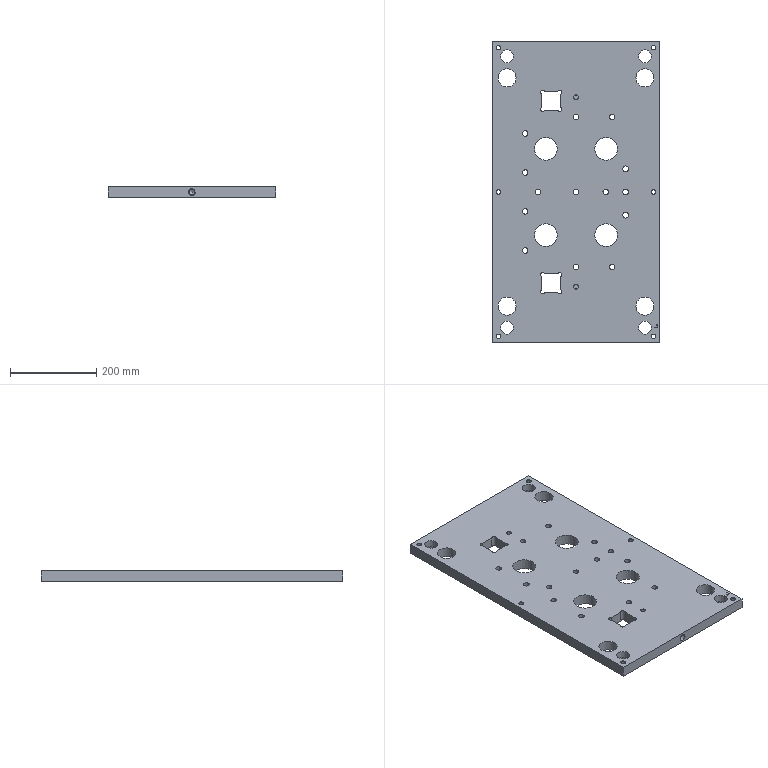Part | NX | features 模具.stp<1>[9] 2 | 1 solid | 153 faces | box 390 x 700 x 25 mm | volume 6189938 mm3 | cylinder 78 | plane 73 | cone 2 | commonest cylinder face diameters 13 x14 18 x14 10 x8 10.5 x8 11.7 x6 12 x6